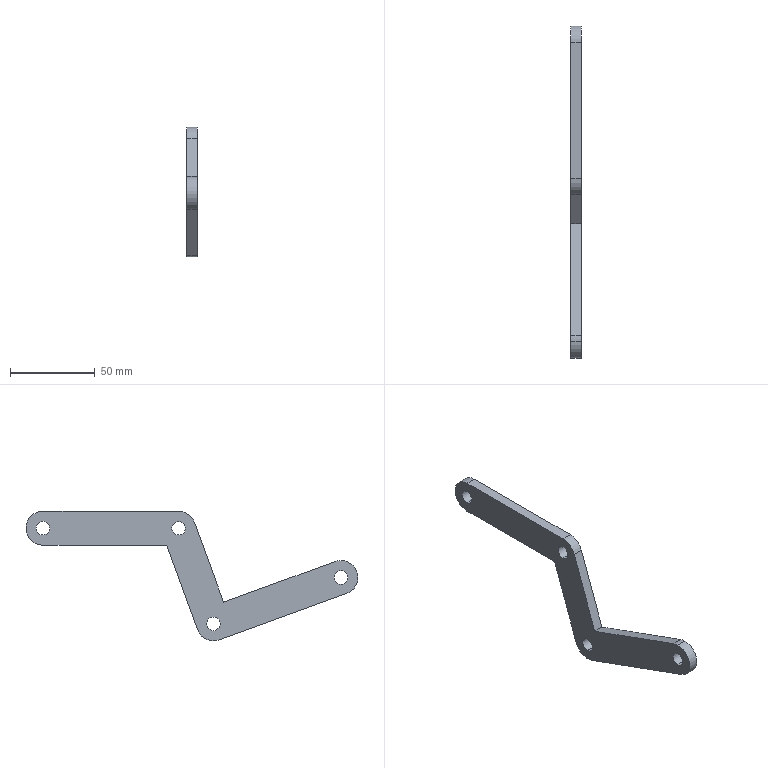Part | SolidWorks | features Extrusion 1 | 1 solid | 21 faces | box 6 x 195.697 x 76.382 mm | volume 26896 mm3 | cylinder 13 | plane 8 | commonest cylinder face diameters 8 x8 20 x5
STEP:
#1=CARTESIAN_POINT('',(6.,80.,4.));
#2=VERTEX_POINT('',#1);
#3=CARTESIAN_POINT('',(6.,80.,-4.));
#4=VERTEX_POINT('',#3);
#5=CARTESIAN_POINT('',(6.,80.,0.));
#6=DIRECTION('',(1.,0.,0.));
#7=DIRECTION('',(0.,0.,-1.));
#8=AXIS2_PLACEMENT_3D('',#5,#6,#7);
#9=CIRCLE('',#8,4.);
#10=EDGE_CURVE('',#2,#4,#9,.T.);
#11=ORIENTED_EDGE('',*,*,#10,.T.);
#12=CARTESIAN_POINT('',(0.,80.,-4.));
#13=VERTEX_POINT('',#12);
#14=CARTESIAN_POINT('',(6.,80.,-4.));
#15=DIRECTION('',(-1.,0.,0.));
#16=VECTOR('',#15,1000.);
#17=LINE('',#14,#16);
#18=EDGE_CURVE('',#4,#13,#17,.T.);
#19=ORIENTED_EDGE('',*,*,#18,.T.);
#20=CARTESIAN_POINT('',(0.,80.,4.));
#21=VERTEX_POINT('',#20);
#22=CARTESIAN_POINT('',(0.,80.,0.));
#23=DIRECTION('',(1.,0.,0.));
#24=DIRECTION('',(0.,0.,-1.));
#25=AXIS2_PLACEMENT_3D('',#22,#23,#24);
#26=CIRCLE('',#25,4.);
#27=EDGE_CURVE('',#21,#13,#26,.T.);
#28=ORIENTED_EDGE('',*,*,#27,.F.);
#29=CARTESIAN_POINT('',(6.,80.,4.));
#30=DIRECTION('',(-1.,0.,0.));
#31=VECTOR('',#30,1000.);
#32=LINE('',#29,#31);
#33=EDGE_CURVE('',#2,#21,#32,.T.);
#34=ORIENTED_EDGE('',*,*,#33,.F.);
#35=EDGE_LOOP('',(#11,#19,#28,#34));
#36=FACE_OUTER_BOUND('',#35,.T.);
#37=CARTESIAN_POINT('',(6.,80.,0.));
#38=DIRECTION('',(-1.,0.,0.));
#39=DIRECTION('',(0.,0.,1.));
#40=AXIS2_PLACEMENT_3D('',#37,#38,#39);
#41=CYLINDRICAL_SURFACE('',#40,4.);
#42=ADVANCED_FACE('',(#36),#41,.F.);
#43=CARTESIAN_POINT('',(6.,-95.697,-25.02));
#44=VERTEX_POINT('',#43);
#45=CARTESIAN_POINT('',(6.,-95.697,-33.02));
#46=VERTEX_POINT('',#45);
#47=CARTESIAN_POINT('',(6.,-95.697,-29.02));
#48=DIRECTION('',(1.,0.,0.));
#49=DIRECTION('',(0.,0.,-1.));
#50=AXIS2_PLACEMENT_3D('',#47,#48,#49);
#51=CIRCLE('',#50,4.);
#52=EDGE_CURVE('',#44,#46,#51,.T.);
#53=ORIENTED_EDGE('',*,*,#52,.T.);
#54=CARTESIAN_POINT('',(0.,-95.697,-33.02));
#55=VERTEX_POINT('',#54);
#56=CARTESIAN_POINT('',(6.,-95.697,-33.02));
#57=DIRECTION('',(-1.,0.,0.));
#58=VECTOR('',#57,1000.);
#59=LINE('',#56,#58);
#60=EDGE_CURVE('',#46,#55,#59,.T.);
#61=ORIENTED_EDGE('',*,*,#60,.T.);
#62=CARTESIAN_POINT('',(0.,-95.697,-25.02));
#63=VERTEX_POINT('',#62);
#64=CARTESIAN_POINT('',(0.,-95.697,-29.02));
#65=DIRECTION('',(1.,0.,0.));
#66=DIRECTION('',(0.,0.,-1.));
#67=AXIS2_PLACEMENT_3D('',#64,#65,#66);
#68=CIRCLE('',#67,4.);
#69=EDGE_CURVE('',#63,#55,#68,.T.);
#70=ORIENTED_EDGE('',*,*,#69,.F.);
#71=CARTESIAN_POINT('',(6.,-95.697,-25.02));
#72=DIRECTION('',(-1.,0.,0.));
#73=VECTOR('',#72,1000.);
#74=LINE('',#71,#73);
#75=EDGE_CURVE('',#44,#63,#74,.T.);
#76=ORIENTED_EDGE('',*,*,#75,.F.);
#77=EDGE_LOOP('',(#53,#61,#70,#76));
#78=FACE_OUTER_BOUND('',#77,.T.);
#79=CARTESIAN_POINT('',(6.,-95.697,-29.02));
#80=DIRECTION('',(-1.,0.,0.));
#81=DIRECTION('',(0.,0.,1.));
#82=AXIS2_PLACEMENT_3D('',#79,#80,#81);
#83=CYLINDRICAL_SURFACE('',#82,4.);
#84=ADVANCED_FACE('',(#78),#83,.F.);
#85=CARTESIAN_POINT('',(6.,-20.521,-52.382));
#86=VERTEX_POINT('',#85);
#87=CARTESIAN_POINT('',(6.,-20.521,-60.382));
#88=VERTEX_POINT('',#87);
#89=CARTESIAN_POINT('',(6.,-20.521,-56.382));
#90=DIRECTION('',(1.,0.,0.));
#91=DIRECTION('',(0.,0.,-1.));
#92=AXIS2_PLACEMENT_3D('',#89,#90,#91);
#93=CIRCLE('',#92,4.);
#94=EDGE_CURVE('',#86,#88,#93,.T.);
#95=ORIENTED_EDGE('',*,*,#94,.T.);
#96=CARTESIAN_POINT('',(0.,-20.521,-60.382));
#97=VERTEX_POINT('',#96);
#98=CARTESIAN_POINT('',(6.,-20.521,-60.382));
#99=DIRECTION('',(-1.,0.,0.));
#100=VECTOR('',#99,1000.);
#101=LINE('',#98,#100);
#102=EDGE_CURVE('',#88,#97,#101,.T.);
#103=ORIENTED_EDGE('',*,*,#102,.T.);
#104=CARTESIAN_POINT('',(0.,-20.521,-52.382));
#105=VERTEX_POINT('',#104);
#106=CARTESIAN_POINT('',(0.,-20.521,-56.382));
#107=DIRECTION('',(1.,0.,0.));
#108=DIRECTION('',(0.,0.,-1.));
#109=AXIS2_PLACEMENT_3D('',#106,#107,#108);
#110=CIRCLE('',#109,4.);
#111=EDGE_CURVE('',#105,#97,#110,.T.);
#112=ORIENTED_EDGE('',*,*,#111,.F.);
#113=CARTESIAN_POINT('',(6.,-20.521,-52.382));
#114=DIRECTION('',(-1.,0.,0.));
#115=VECTOR('',#114,1000.);
#116=LINE('',#113,#115);
#117=EDGE_CURVE('',#86,#105,#116,.T.);
#118=ORIENTED_EDGE('',*,*,#117,.F.);
#119=EDGE_LOOP('',(#95,#103,#112,#118));
#120=FACE_OUTER_BOUND('',#119,.T.);
#121=CARTESIAN_POINT('',(6.,-20.521,-56.382));
#122=DIRECTION('',(-1.,0.,0.));
#123=DIRECTION('',(0.,0.,1.));
#124=AXIS2_PLACEMENT_3D('',#121,#122,#123);
#125=CYLINDRICAL_SURFACE('',#124,4.);
#126=ADVANCED_FACE('',(#120),#125,.F.);
#127=CARTESIAN_POINT('',(6.,0.,4.));
#128=VERTEX_POINT('',#127);
#129=CARTESIAN_POINT('',(6.,0.,-4.));
#130=VERTEX_POINT('',#129);
#131=CARTESIAN_POINT('',(6.,0.,0.));
#132=DIRECTION('',(1.,0.,0.));
#133=DIRECTION('',(0.,0.,-1.));
#134=AXIS2_PLACEMENT_3D('',#131,#132,#133);
#135=CIRCLE('',#134,4.);
#136=EDGE_CURVE('',#128,#130,#135,.T.);
#137=ORIENTED_EDGE('',*,*,#136,.T.);
#138=CARTESIAN_POINT('',(0.,0.,-4.));
#139=VERTEX_POINT('',#138);
#140=CARTESIAN_POINT('',(6.,0.,-4.));
#141=DIRECTION('',(-1.,0.,0.));
#142=VECTOR('',#141,1000.);
#143=LINE('',#140,#142);
#144=EDGE_CURVE('',#130,#139,#143,.T.);
#145=ORIENTED_EDGE('',*,*,#144,.T.);
#146=CARTESIAN_POINT('',(0.,0.,4.));
#147=VERTEX_POINT('',#146);
#148=CARTESIAN_POINT('',(0.,0.,0.));
#149=DIRECTION('',(1.,0.,0.));
#150=DIRECTION('',(0.,0.,-1.));
#151=AXIS2_PLACEMENT_3D('',#148,#149,#150);
#152=CIRCLE('',#151,4.);
#153=EDGE_CURVE('',#147,#139,#152,.T.);
#154=ORIENTED_EDGE('',*,*,#153,.F.);
#155=CARTESIAN_POINT('',(6.,0.,4.));
#156=DIRECTION('',(-1.,0.,0.));
#157=VECTOR('',#156,1000.);
#158=LINE('',#155,#157);
#159=EDGE_CURVE('',#128,#147,#158,.T.);
#160=ORIENTED_EDGE('',*,*,#159,.F.);
#161=EDGE_LOOP('',(#137,#145,#154,#160));
#162=FACE_OUTER_BOUND('',#161,.T.);
#163=CARTESIAN_POINT('',(6.,0.,0.));
#164=DIRECTION('',(-1.,0.,0.));
#165=DIRECTION('',(0.,0.,1.));
#166=AXIS2_PLACEMENT_3D('',#163,#164,#165);
#167=CYLINDRICAL_SURFACE('',#166,4.);
#168=ADVANCED_FACE('',(#162),#167,.F.);
#169=CARTESIAN_POINT('',(6.,-95.697,-19.02));
#170=VERTEX_POINT('',#169);
#171=CARTESIAN_POINT('',(6.,-99.117,-38.417));
#172=VERTEX_POINT('',#171);
#173=CARTESIAN_POINT('',(6.,-95.697,-29.02));
#174=DIRECTION('',(1.,0.,0.));
#175=DIRECTION('',(0.,0.,-1.));
#176=AXIS2_PLACEMENT_3D('',#173,#174,#175);
#177=CIRCLE('',#176,10.);
#178=EDGE_CURVE('',#170,#172,#177,.T.);
#179=ORIENTED_EDGE('',*,*,#178,.F.);
#180=CARTESIAN_POINT('',(0.,-95.697,-19.02));
#181=VERTEX_POINT('',#180);
#182=CARTESIAN_POINT('',(6.,-95.697,-19.02));
#183=DIRECTION('',(-1.,0.,0.));
#184=VECTOR('',#183,1000.);
#185=LINE('',#182,#184);
#186=EDGE_CURVE('',#170,#181,#185,.T.);
#187=ORIENTED_EDGE('',*,*,#186,.T.);
#188=CARTESIAN_POINT('',(0.,-99.117,-38.417));
#189=VERTEX_POINT('',#188);
#190=CARTESIAN_POINT('',(0.,-95.697,-29.02));
#191=DIRECTION('',(1.,0.,0.));
#192=DIRECTION('',(0.,0.,-1.));
#193=AXIS2_PLACEMENT_3D('',#190,#191,#192);
#194=CIRCLE('',#193,10.);
#195=EDGE_CURVE('',#181,#189,#194,.T.);
#196=ORIENTED_EDGE('',*,*,#195,.T.);
#197=CARTESIAN_POINT('',(6.,-99.117,-38.417));
#198=DIRECTION('',(-1.,0.,0.));
#199=VECTOR('',#198,1000.);
#200=LINE('',#197,#199);
#201=EDGE_CURVE('',#172,#189,#200,.T.);
#202=ORIENTED_EDGE('',*,*,#201,.F.);
#203=EDGE_LOOP('',(#179,#187,#196,#202));
#204=FACE_OUTER_BOUND('',#203,.T.);
#205=CARTESIAN_POINT('',(6.,-95.697,-29.02));
#206=DIRECTION('',(-1.,0.,0.));
#207=DIRECTION('',(0.,0.,1.));
#208=AXIS2_PLACEMENT_3D('',#205,#206,#207);
#209=CYLINDRICAL_SURFACE('',#208,10.);
#210=ADVANCED_FACE('',(#204),#209,.T.);
#211=CARTESIAN_POINT('',(0.,7.002,-10.));
#212=VERTEX_POINT('',#211);
#213=CARTESIAN_POINT('',(0.,-11.124,-59.802));
#214=VERTEX_POINT('',#213);
#215=CARTESIAN_POINT('',(0.,9.397,-3.42));
#216=DIRECTION('',(0.,-0.342,-0.9397));
#217=VECTOR('',#216,1000.);
#218=LINE('',#215,#217);
#219=EDGE_CURVE('',#212,#214,#218,.T.);
#220=ORIENTED_EDGE('',*,*,#219,.F.);
#221=CARTESIAN_POINT('',(6.,7.002,-10.));
#222=VERTEX_POINT('',#221);
#223=CARTESIAN_POINT('',(6.,7.002,-10.));
#224=DIRECTION('',(-1.,0.,0.));
#225=VECTOR('',#224,1000.);
#226=LINE('',#223,#225);
#227=EDGE_CURVE('',#222,#212,#226,.T.);
#228=ORIENTED_EDGE('',*,*,#227,.F.);
#229=CARTESIAN_POINT('',(6.,-11.124,-59.802));
#230=VERTEX_POINT('',#229);
#231=CARTESIAN_POINT('',(6.,9.397,-3.42));
#232=DIRECTION('',(0.,-0.342,-0.9397));
#233=VECTOR('',#232,1000.);
#234=LINE('',#231,#233);
#235=EDGE_CURVE('',#222,#230,#234,.T.);
#236=ORIENTED_EDGE('',*,*,#235,.T.);
#237=CARTESIAN_POINT('',(6.,-11.124,-59.802));
#238=DIRECTION('',(-1.,0.,0.));
#239=VECTOR('',#238,1000.);
#240=LINE('',#237,#239);
#241=EDGE_CURVE('',#230,#214,#240,.T.);
#242=ORIENTED_EDGE('',*,*,#241,.T.);
#243=EDGE_LOOP('',(#220,#228,#236,#242));
#244=FACE_OUTER_BOUND('',#243,.T.);
#245=CARTESIAN_POINT('',(6.,9.397,-3.42));
#246=DIRECTION('',(0.,0.9397,-0.342));
#247=DIRECTION('',(0.,0.342,0.9397));
#248=AXIS2_PLACEMENT_3D('',#245,#246,#247);
#249=PLANE('',#248);
#250=ADVANCED_FACE('',(#244),#249,.T.);
#251=CARTESIAN_POINT('',(0.,80.,-10.));
#252=VERTEX_POINT('',#251);
#253=CARTESIAN_POINT('',(0.,0.,-10.));
#254=DIRECTION('',(0.,-1.,0.));
#255=VECTOR('',#254,1000.);
#256=LINE('',#253,#255);
#257=EDGE_CURVE('',#252,#212,#256,.T.);
#258=ORIENTED_EDGE('',*,*,#257,.F.);
#259=CARTESIAN_POINT('',(6.,80.,-10.));
#260=VERTEX_POINT('',#259);
#261=CARTESIAN_POINT('',(6.,80.,-10.));
#262=DIRECTION('',(-1.,0.,0.));
#263=VECTOR('',#262,1000.);
#264=LINE('',#261,#263);
#265=EDGE_CURVE('',#260,#252,#264,.T.);
#266=ORIENTED_EDGE('',*,*,#265,.F.);
#267=CARTESIAN_POINT('',(6.,0.,-10.));
#268=DIRECTION('',(0.,-1.,0.));
#269=VECTOR('',#268,1000.);
#270=LINE('',#267,#269);
#271=EDGE_CURVE('',#260,#222,#270,.T.);
#272=ORIENTED_EDGE('',*,*,#271,.T.);
#273=ORIENTED_EDGE('',*,*,#227,.T.);
#274=EDGE_LOOP('',(#258,#266,#272,#273));
#275=FACE_OUTER_BOUND('',#274,.T.);
#276=CARTESIAN_POINT('',(6.,0.,-10.));
#277=DIRECTION('',(0.,0.,-1.));
#278=DIRECTION('',(0.,1.,0.));
#279=AXIS2_PLACEMENT_3D('',#276,#277,#278);
#280=PLANE('',#279);
#281=ADVANCED_FACE('',(#275),#280,.T.);
#282=CARTESIAN_POINT('',(0.,80.,10.));
#283=VERTEX_POINT('',#282);
#284=CARTESIAN_POINT('',(0.,80.,0.));
#285=DIRECTION('',(1.,0.,0.));
#286=DIRECTION('',(0.,0.,-1.));
#287=AXIS2_PLACEMENT_3D('',#284,#285,#286);
#288=CIRCLE('',#287,10.);
#289=EDGE_CURVE('',#252,#283,#288,.T.);
#290=ORIENTED_EDGE('',*,*,#289,.T.);
#291=CARTESIAN_POINT('',(6.,80.,10.));
#292=VERTEX_POINT('',#291);
#293=CARTESIAN_POINT('',(6.,80.,10.));
#294=DIRECTION('',(-1.,0.,0.));
#295=VECTOR('',#294,1000.);
#296=LINE('',#293,#295);
#297=EDGE_CURVE('',#292,#283,#296,.T.);
#298=ORIENTED_EDGE('',*,*,#297,.F.);
#299=CARTESIAN_POINT('',(6.,80.,0.));
#300=DIRECTION('',(1.,0.,0.));
#301=DIRECTION('',(0.,0.,-1.));
#302=AXIS2_PLACEMENT_3D('',#299,#300,#301);
#303=CIRCLE('',#302,10.);
#304=EDGE_CURVE('',#260,#292,#303,.T.);
#305=ORIENTED_EDGE('',*,*,#304,.F.);
#306=ORIENTED_EDGE('',*,*,#265,.T.);
#307=EDGE_LOOP('',(#290,#298,#305,#306));
#308=FACE_OUTER_BOUND('',#307,.T.);
#309=CARTESIAN_POINT('',(6.,80.,0.));
#310=DIRECTION('',(-1.,0.,0.));
#311=DIRECTION('',(0.,0.,1.));
#312=AXIS2_PLACEMENT_3D('',#309,#310,#311);
#313=CYLINDRICAL_SURFACE('',#312,10.);
#314=ADVANCED_FACE('',(#308),#313,.T.);
#315=CARTESIAN_POINT('',(0.,0.,10.));
#316=VERTEX_POINT('',#315);
#317=CARTESIAN_POINT('',(0.,0.,10.));
#318=DIRECTION('',(0.,-1.,0.));
#319=VECTOR('',#318,1000.);
#320=LINE('',#317,#319);
#321=EDGE_CURVE('',#283,#316,#320,.T.);
#322=ORIENTED_EDGE('',*,*,#321,.T.);
#323=CARTESIAN_POINT('',(6.,0.,10.));
#324=VERTEX_POINT('',#323);
#325=CARTESIAN_POINT('',(6.,0.,10.));
#326=DIRECTION('',(-1.,0.,0.));
#327=VECTOR('',#326,1000.);
#328=LINE('',#325,#327);
#329=EDGE_CURVE('',#324,#316,#328,.T.);
#330=ORIENTED_EDGE('',*,*,#329,.F.);
#331=CARTESIAN_POINT('',(6.,0.,10.));
#332=DIRECTION('',(0.,-1.,0.));
#333=VECTOR('',#332,1000.);
#334=LINE('',#331,#333);
#335=EDGE_CURVE('',#292,#324,#334,.T.);
#336=ORIENTED_EDGE('',*,*,#335,.F.);
#337=ORIENTED_EDGE('',*,*,#297,.T.);
#338=EDGE_LOOP('',(#322,#330,#336,#337));
#339=FACE_OUTER_BOUND('',#338,.T.);
#340=CARTESIAN_POINT('',(6.,0.,10.));
#341=DIRECTION('',(0.,0.,-1.));
#342=DIRECTION('',(0.,1.,0.));
#343=AXIS2_PLACEMENT_3D('',#340,#341,#342);
#344=PLANE('',#343);
#345=ADVANCED_FACE('',(#339),#344,.F.);
#346=CARTESIAN_POINT('',(0.,-9.397,3.42));
#347=VERTEX_POINT('',#346);
#348=CARTESIAN_POINT('',(0.,0.,0.));
#349=DIRECTION('',(1.,0.,0.));
#350=DIRECTION('',(0.,0.,-1.));
#351=AXIS2_PLACEMENT_3D('',#348,#349,#350);
#352=CIRCLE('',#351,10.);
#353=EDGE_CURVE('',#316,#347,#352,.T.);
#354=ORIENTED_EDGE('',*,*,#353,.T.);
#355=CARTESIAN_POINT('',(6.,-9.397,3.42));
#356=VERTEX_POINT('',#355);
#357=CARTESIAN_POINT('',(6.,-9.397,3.42));
#358=DIRECTION('',(-1.,0.,0.));
#359=VECTOR('',#358,1000.);
#360=LINE('',#357,#359);
#361=EDGE_CURVE('',#356,#347,#360,.T.);
#362=ORIENTED_EDGE('',*,*,#361,.F.);
#363=CARTESIAN_POINT('',(6.,0.,0.));
#364=DIRECTION('',(1.,0.,0.));
#365=DIRECTION('',(0.,0.,-1.));
#366=AXIS2_PLACEMENT_3D('',#363,#364,#365);
#367=CIRCLE('',#366,10.);
#368=EDGE_CURVE('',#324,#356,#367,.T.);
#369=ORIENTED_EDGE('',*,*,#368,.F.);
#370=ORIENTED_EDGE('',*,*,#329,.T.);
#371=EDGE_LOOP('',(#354,#362,#369,#370));
#372=FACE_OUTER_BOUND('',#371,.T.);
#373=CARTESIAN_POINT('',(6.,0.,0.));
#374=DIRECTION('',(-1.,0.,0.));
#375=DIRECTION('',(0.,0.,1.));
#376=AXIS2_PLACEMENT_3D('',#373,#374,#375);
#377=CYLINDRICAL_SURFACE('',#376,10.);
#378=ADVANCED_FACE('',(#372),#377,.T.);
#379=CARTESIAN_POINT('',(0.,-26.498,-43.564));
#380=VERTEX_POINT('',#379);
#381=CARTESIAN_POINT('',(0.,-9.397,3.42));
#382=DIRECTION('',(0.,-0.342,-0.9397));
#383=VECTOR('',#382,1000.);
#384=LINE('',#381,#383);
#385=EDGE_CURVE('',#347,#380,#384,.T.);
#386=ORIENTED_EDGE('',*,*,#385,.T.);
#387=CARTESIAN_POINT('',(6.,-26.498,-43.564));
#388=VERTEX_POINT('',#387);
#389=CARTESIAN_POINT('',(6.,-26.498,-43.564));
#390=DIRECTION('',(-1.,0.,0.));
#391=VECTOR('',#390,1000.);
#392=LINE('',#389,#391);
#393=EDGE_CURVE('',#388,#380,#392,.T.);
#394=ORIENTED_EDGE('',*,*,#393,.F.);
#395=CARTESIAN_POINT('',(6.,-9.397,3.42));
#396=DIRECTION('',(0.,-0.342,-0.9397));
#397=VECTOR('',#396,1000.);
#398=LINE('',#395,#397);
#399=EDGE_CURVE('',#356,#388,#398,.T.);
#400=ORIENTED_EDGE('',*,*,#399,.F.);
#401=ORIENTED_EDGE('',*,*,#361,.T.);
#402=EDGE_LOOP('',(#386,#394,#400,#401));
#403=FACE_OUTER_BOUND('',#402,.T.);
#404=CARTESIAN_POINT('',(6.,-9.397,3.42));
#405=DIRECTION('',(0.,0.9397,-0.342));
#406=DIRECTION('',(0.,0.342,0.9397));
#407=AXIS2_PLACEMENT_3D('',#404,#405,#406);
#408=PLANE('',#407);
#409=ADVANCED_FACE('',(#403),#408,.F.);
#410=CARTESIAN_POINT('',(0.,-92.276,-19.623));
#411=VERTEX_POINT('',#410);
#412=CARTESIAN_POINT('',(0.,-17.101,-46.985));
#413=DIRECTION('',(0.,-0.9397,0.342));
#414=VECTOR('',#413,1000.);
#415=LINE('',#412,#414);
#416=EDGE_CURVE('',#380,#411,#415,.T.);
#417=ORIENTED_EDGE('',*,*,#416,.T.);
#418=CARTESIAN_POINT('',(6.,-92.276,-19.623));
#419=VERTEX_POINT('',#418);
#420=CARTESIAN_POINT('',(6.,-92.276,-19.623));
#421=DIRECTION('',(-1.,0.,0.));
#422=VECTOR('',#421,1000.);
#423=LINE('',#420,#422);
#424=EDGE_CURVE('',#419,#411,#423,.T.);
#425=ORIENTED_EDGE('',*,*,#424,.F.);
#426=CARTESIAN_POINT('',(6.,-17.101,-46.985));
#427=DIRECTION('',(0.,-0.9397,0.342));
#428=VECTOR('',#427,1000.);
#429=LINE('',#426,#428);
#430=EDGE_CURVE('',#388,#419,#429,.T.);
#431=ORIENTED_EDGE('',*,*,#430,.F.);
#432=ORIENTED_EDGE('',*,*,#393,.T.);
#433=EDGE_LOOP('',(#417,#425,#431,#432));
#434=FACE_OUTER_BOUND('',#433,.T.);
#435=CARTESIAN_POINT('',(6.,-17.101,-46.985));
#436=DIRECTION('',(0.,-0.342,-0.9397));
#437=DIRECTION('',(0.,0.9397,-0.342));
#438=AXIS2_PLACEMENT_3D('',#435,#436,#437);
#439=PLANE('',#438);
#440=ADVANCED_FACE('',(#434),#439,.F.);
#441=ORIENTED_EDGE('',*,*,#186,.F.);
#442=CARTESIAN_POINT('',(6.,-95.697,-29.02));
#443=DIRECTION('',(1.,0.,0.));
#444=DIRECTION('',(0.,0.,-1.));
#445=AXIS2_PLACEMENT_3D('',#442,#443,#444);
#446=CIRCLE('',#445,10.);
#447=EDGE_CURVE('',#419,#170,#446,.T.);
#448=ORIENTED_EDGE('',*,*,#447,.F.);
#449=ORIENTED_EDGE('',*,*,#424,.T.);
#450=CARTESIAN_POINT('',(0.,-95.697,-29.02));
#451=DIRECTION('',(1.,0.,0.));
#452=DIRECTION('',(0.,0.,-1.));
#453=AXIS2_PLACEMENT_3D('',#450,#451,#452);
#454=CIRCLE('',#453,10.);
#455=EDGE_CURVE('',#411,#181,#454,.T.);
#456=ORIENTED_EDGE('',*,*,#455,.T.);
#457=EDGE_LOOP('',(#441,#448,#449,#456));
#458=FACE_OUTER_BOUND('',#457,.T.);
#459=CARTESIAN_POINT('',(6.,-95.697,-29.02));
#460=DIRECTION('',(-1.,0.,0.));
#461=DIRECTION('',(0.,0.,1.));
#462=AXIS2_PLACEMENT_3D('',#459,#460,#461);
#463=CYLINDRICAL_SURFACE('',#462,10.);
#464=ADVANCED_FACE('',(#458),#463,.T.);
#465=CARTESIAN_POINT('',(0.,-23.941,-65.778));
#466=VERTEX_POINT('',#465);
#467=CARTESIAN_POINT('',(0.,-23.941,-65.778));
#468=DIRECTION('',(0.,-0.9397,0.342));
#469=VECTOR('',#468,1000.);
#470=LINE('',#467,#469);
#471=EDGE_CURVE('',#466,#189,#470,.T.);
#472=ORIENTED_EDGE('',*,*,#471,.F.);
#473=CARTESIAN_POINT('',(6.,-23.941,-65.778));
#474=VERTEX_POINT('',#473);
#475=CARTESIAN_POINT('',(6.,-23.941,-65.778));
#476=DIRECTION('',(-1.,0.,0.));
#477=VECTOR('',#476,1000.);
#478=LINE('',#475,#477);
#479=EDGE_CURVE('',#474,#466,#478,.T.);
#480=ORIENTED_EDGE('',*,*,#479,.F.);
#481=CARTESIAN_POINT('',(6.,-23.941,-65.778));
#482=DIRECTION('',(0.,-0.9397,0.342));
#483=VECTOR('',#482,1000.);
#484=LINE('',#481,#483);
#485=EDGE_CURVE('',#474,#172,#484,.T.);
#486=ORIENTED_EDGE('',*,*,#485,.T.);
#487=ORIENTED_EDGE('',*,*,#201,.T.);
#488=EDGE_LOOP('',(#472,#480,#486,#487));
#489=FACE_OUTER_BOUND('',#488,.T.);
#490=CARTESIAN_POINT('',(6.,-23.941,-65.778));
#491=DIRECTION('',(0.,-0.342,-0.9397));
#492=DIRECTION('',(0.,0.9397,-0.342));
#493=AXIS2_PLACEMENT_3D('',#490,#491,#492);
#494=PLANE('',#493);
#495=ADVANCED_FACE('',(#489),#494,.T.);
#496=ORIENTED_EDGE('',*,*,#144,.F.);
#497=CARTESIAN_POINT('',(6.,0.,0.));
#498=DIRECTION('',(1.,0.,0.));
#499=DIRECTION('',(0.,0.,-1.));
#500=AXIS2_PLACEMENT_3D('',#497,#498,#499);
#501=CIRCLE('',#500,4.);
#502=EDGE_CURVE('',#130,#128,#501,.T.);
#503=ORIENTED_EDGE('',*,*,#502,.T.);
#504=ORIENTED_EDGE('',*,*,#159,.T.);
#505=CARTESIAN_POINT('',(0.,0.,0.));
#506=DIRECTION('',(1.,0.,0.));
#507=DIRECTION('',(0.,0.,-1.));
#508=AXIS2_PLACEMENT_3D('',#505,#506,#507);
#509=CIRCLE('',#508,4.);
#510=EDGE_CURVE('',#139,#147,#509,.T.);
#511=ORIENTED_EDGE('',*,*,#510,.F.);
#512=EDGE_LOOP('',(#496,#503,#504,#511));
#513=FACE_OUTER_BOUND('',#512,.T.);
#514=CARTESIAN_POINT('',(6.,0.,0.));
#515=DIRECTION('',(-1.,0.,0.));
#516=DIRECTION('',(0.,0.,1.));
#517=AXIS2_PLACEMENT_3D('',#514,#515,#516);
#518=CYLINDRICAL_SURFACE('',#517,4.);
#519=ADVANCED_FACE('',(#513),#518,.F.);
#520=ORIENTED_EDGE('',*,*,#102,.F.);
#521=CARTESIAN_POINT('',(6.,-20.521,-56.382));
#522=DIRECTION('',(1.,0.,0.));
#523=DIRECTION('',(0.,0.,-1.));
#524=AXIS2_PLACEMENT_3D('',#521,#522,#523);
#525=CIRCLE('',#524,4.);
#526=EDGE_CURVE('',#88,#86,#525,.T.);
#527=ORIENTED_EDGE('',*,*,#526,.T.);
#528=ORIENTED_EDGE('',*,*,#117,.T.);
#529=CARTESIAN_POINT('',(0.,-20.521,-56.382));
#530=DIRECTION('',(1.,0.,0.));
#531=DIRECTION('',(0.,0.,-1.));
#532=AXIS2_PLACEMENT_3D('',#529,#530,#531);
#533=CIRCLE('',#532,4.);
#534=EDGE_CURVE('',#97,#105,#533,.T.);
#535=ORIENTED_EDGE('',*,*,#534,.F.);
#536=EDGE_LOOP('',(#520,#527,#528,#535));
#537=FACE_OUTER_BOUND('',#536,.T.);
#538=CARTESIAN_POINT('',(6.,-20.521,-56.382));
#539=DIRECTION('',(-1.,0.,0.));
#540=DIRECTION('',(0.,0.,1.));
#541=AXIS2_PLACEMENT_3D('',#538,#539,#540);
#542=CYLINDRICAL_SURFACE('',#541,4.);
#543=ADVANCED_FACE('',(#537),#542,.F.);
#544=ORIENTED_EDGE('',*,*,#60,.F.);
#545=CARTESIAN_POINT('',(6.,-95.697,-29.02));
#546=DIRECTION('',(1.,0.,0.));
#547=DIRECTION('',(0.,0.,-1.));
#548=AXIS2_PLACEMENT_3D('',#545,#546,#547);
#549=CIRCLE('',#548,4.);
#550=EDGE_CURVE('',#46,#44,#549,.T.);
#551=ORIENTED_EDGE('',*,*,#550,.T.);
#552=ORIENTED_EDGE('',*,*,#75,.T.);
#553=CARTESIAN_POINT('',(0.,-95.697,-29.02));
#554=DIRECTION('',(1.,0.,0.));
#555=DIRECTION('',(0.,0.,-1.));
#556=AXIS2_PLACEMENT_3D('',#553,#554,#555);
#557=CIRCLE('',#556,4.);
#558=EDGE_CURVE('',#55,#63,#557,.T.);
#559=ORIENTED_EDGE('',*,*,#558,.F.);
#560=EDGE_LOOP('',(#544,#551,#552,#559));
#561=FACE_OUTER_BOUND('',#560,.T.);
#562=CARTESIAN_POINT('',(6.,-95.697,-29.02));
#563=DIRECTION('',(-1.,0.,0.));
#564=DIRECTION('',(0.,0.,1.));
#565=AXIS2_PLACEMENT_3D('',#562,#563,#564);
#566=CYLINDRICAL_SURFACE('',#565,4.);
#567=ADVANCED_FACE('',(#561),#566,.F.);
#568=CARTESIAN_POINT('',(0.,-20.521,-56.382));
#569=DIRECTION('',(1.,0.,0.));
#570=DIRECTION('',(0.,0.,-1.));
#571=AXIS2_PLACEMENT_3D('',#568,#569,#570);
#572=CIRCLE('',#571,10.);
#573=EDGE_CURVE('',#466,#214,#572,.T.);
#574=ORIENTED_EDGE('',*,*,#573,.T.);
#575=ORIENTED_EDGE('',*,*,#241,.F.);
#576=CARTESIAN_POINT('',(6.,-20.521,-56.382));
#577=DIRECTION('',(1.,0.,0.));
#578=DIRECTION('',(0.,0.,-1.));
#579=AXIS2_PLACEMENT_3D('',#576,#577,#578);
#580=CIRCLE('',#579,10.);
#581=EDGE_CURVE('',#474,#230,#580,.T.);
#582=ORIENTED_EDGE('',*,*,#581,.F.);
#583=ORIENTED_EDGE('',*,*,#479,.T.);
#584=EDGE_LOOP('',(#574,#575,#582,#583));
#585=FACE_OUTER_BOUND('',#584,.T.);
#586=CARTESIAN_POINT('',(6.,-20.521,-56.382));
#587=DIRECTION('',(-1.,0.,0.));
#588=DIRECTION('',(0.,0.,1.));
#589=AXIS2_PLACEMENT_3D('',#586,#587,#588);
#590=CYLINDRICAL_SURFACE('',#589,10.);
#591=ADVANCED_FACE('',(#585),#590,.T.);
#592=ORIENTED_EDGE('',*,*,#18,.F.);
#593=CARTESIAN_POINT('',(6.,80.,0.));
#594=DIRECTION('',(1.,0.,0.));
#595=DIRECTION('',(0.,0.,-1.));
#596=AXIS2_PLACEMENT_3D('',#593,#594,#595);
#597=CIRCLE('',#596,4.);
#598=EDGE_CURVE('',#4,#2,#597,.T.);
#599=ORIENTED_EDGE('',*,*,#598,.T.);
#600=ORIENTED_EDGE('',*,*,#33,.T.);
#601=CARTESIAN_POINT('',(0.,80.,0.));
#602=DIRECTION('',(1.,0.,0.));
#603=DIRECTION('',(0.,0.,-1.));
#604=AXIS2_PLACEMENT_3D('',#601,#602,#603);
#605=CIRCLE('',#604,4.);
#606=EDGE_CURVE('',#13,#21,#605,.T.);
#607=ORIENTED_EDGE('',*,*,#606,.F.);
#608=EDGE_LOOP('',(#592,#599,#600,#607));
#609=FACE_OUTER_BOUND('',#608,.T.);
#610=CARTESIAN_POINT('',(6.,80.,0.));
#611=DIRECTION('',(-1.,0.,0.));
#612=DIRECTION('',(0.,0.,1.));
#613=AXIS2_PLACEMENT_3D('',#610,#611,#612);
#614=CYLINDRICAL_SURFACE('',#613,4.);
#615=ADVANCED_FACE('',(#609),#614,.F.);
#616=ORIENTED_EDGE('',*,*,#235,.F.);
#617=ORIENTED_EDGE('',*,*,#271,.F.);
#618=ORIENTED_EDGE('',*,*,#304,.T.);
#619=ORIENTED_EDGE('',*,*,#335,.T.);
#620=ORIENTED_EDGE('',*,*,#368,.T.);
#621=ORIENTED_EDGE('',*,*,#399,.T.);
#622=ORIENTED_EDGE('',*,*,#430,.T.);
#623=ORIENTED_EDGE('',*,*,#447,.T.);
#624=ORIENTED_EDGE('',*,*,#178,.T.);
#625=ORIENTED_EDGE('',*,*,#485,.F.);
#626=ORIENTED_EDGE('',*,*,#581,.T.);
#627=EDGE_LOOP('',(#616,#617,#618,#619,#620,#621,#622,#623,#624,#625,#626));
#628=FACE_OUTER_BOUND('',#627,.T.);
#629=ORIENTED_EDGE('',*,*,#52,.F.);
#630=ORIENTED_EDGE('',*,*,#550,.F.);
#631=EDGE_LOOP('',(#629,#630));
#632=FACE_BOUND('',#631,.T.);
#633=ORIENTED_EDGE('',*,*,#94,.F.);
#634=ORIENTED_EDGE('',*,*,#526,.F.);
#635=EDGE_LOOP('',(#633,#634));
#636=FACE_BOUND('',#635,.T.);
#637=ORIENTED_EDGE('',*,*,#136,.F.);
#638=ORIENTED_EDGE('',*,*,#502,.F.);
#639=EDGE_LOOP('',(#637,#638));
#640=FACE_BOUND('',#639,.T.);
#641=ORIENTED_EDGE('',*,*,#10,.F.);
#642=ORIENTED_EDGE('',*,*,#598,.F.);
#643=EDGE_LOOP('',(#641,#642));
#644=FACE_BOUND('',#643,.T.);
#645=CARTESIAN_POINT('',(6.,0.,0.));
#646=DIRECTION('',(1.,0.,0.));
#647=DIRECTION('',(0.,0.,-1.));
#648=AXIS2_PLACEMENT_3D('',#645,#646,#647);
#649=PLANE('',#648);
#650=ADVANCED_FACE('',(#628,#632,#636,#640,#644),#649,.T.);
#651=ORIENTED_EDGE('',*,*,#219,.T.);
#652=ORIENTED_EDGE('',*,*,#573,.F.);
#653=ORIENTED_EDGE('',*,*,#471,.T.);
#654=ORIENTED_EDGE('',*,*,#195,.F.);
#655=ORIENTED_EDGE('',*,*,#455,.F.);
#656=ORIENTED_EDGE('',*,*,#416,.F.);
#657=ORIENTED_EDGE('',*,*,#385,.F.);
#658=ORIENTED_EDGE('',*,*,#353,.F.);
#659=ORIENTED_EDGE('',*,*,#321,.F.);
#660=ORIENTED_EDGE('',*,*,#289,.F.);
#661=ORIENTED_EDGE('',*,*,#257,.T.);
#662=EDGE_LOOP('',(#651,#652,#653,#654,#655,#656,#657,#658,#659,#660,#661));
#663=FACE_OUTER_BOUND('',#662,.T.);
#664=ORIENTED_EDGE('',*,*,#69,.T.);
#665=ORIENTED_EDGE('',*,*,#558,.T.);
#666=EDGE_LOOP('',(#664,#665));
#667=FACE_BOUND('',#666,.T.);
#668=ORIENTED_EDGE('',*,*,#111,.T.);
#669=ORIENTED_EDGE('',*,*,#534,.T.);
#670=EDGE_LOOP('',(#668,#669));
#671=FACE_BOUND('',#670,.T.);
#672=ORIENTED_EDGE('',*,*,#153,.T.);
#673=ORIENTED_EDGE('',*,*,#510,.T.);
#674=EDGE_LOOP('',(#672,#673));
#675=FACE_BOUND('',#674,.T.);
#676=ORIENTED_EDGE('',*,*,#27,.T.);
#677=ORIENTED_EDGE('',*,*,#606,.T.);
#678=EDGE_LOOP('',(#676,#677));
#679=FACE_BOUND('',#678,.T.);
#680=CARTESIAN_POINT('',(0.,0.,0.));
#681=DIRECTION('',(1.,0.,0.));
#682=DIRECTION('',(0.,0.,-1.));
#683=AXIS2_PLACEMENT_3D('',#680,#681,#682);
#684=PLANE('',#683);
#685=ADVANCED_FACE('',(#663,#667,#671,#675,#679),#684,.F.);
#686=CLOSED_SHELL('',(#42,#84,#126,#168,#210,#250,#281,#314,#345,#378,#409,#440,#464,#495,#519,#543,#567,#591,#615,#650,#685));
#687=MANIFOLD_SOLID_BREP('',#686);
#688=CARTESIAN_POINT('',(0.,0.,0.));
#689=DIRECTION('',(0.,0.,1.));
#690=DIRECTION('',(1.,0.,0.));
#691=AXIS2_PLACEMENT_3D('',#688,#689,#690);
#692=(LENGTH_UNIT()NAMED_UNIT(*)SI_UNIT(.MILLI.,.METRE.));
#693=UNCERTAINTY_MEASURE_WITH_UNIT(LENGTH_MEASURE(0.00001),#692,'','');
#694=(NAMED_UNIT(*)PLANE_ANGLE_UNIT()SI_UNIT($,.RADIAN.));
#695=(NAMED_UNIT(*)SI_UNIT($,.STERADIAN.)SOLID_ANGLE_UNIT());
#696=(GEOMETRIC_REPRESENTATION_CONTEXT(3)GLOBAL_UNCERTAINTY_ASSIGNED_CONTEXT((#693))GLOBAL_UNIT_ASSIGNED_CONTEXT((#692,#694,#695))REPRESENTATION_CONTEXT('',''));
#697=ADVANCED_BREP_SHAPE_REPRESENTATION('',(#687,#691),#696);